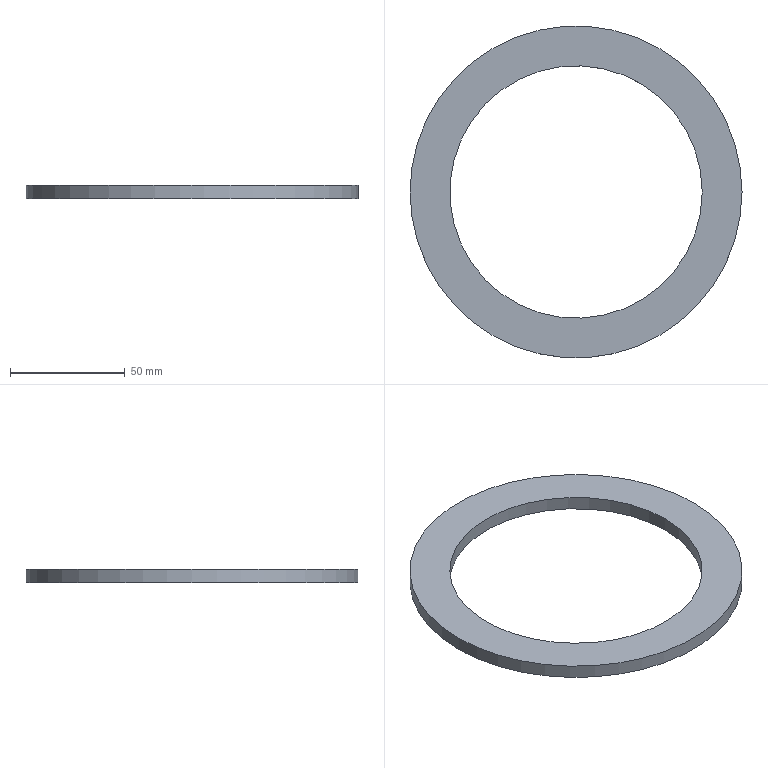Part | NX | features BREP 1 | 1 solid | 4 faces | box 144.7 x 144.7 x 6 mm | volume 41649 mm3 | cylinder 2 | plane 2 | commonest cylinder face diameters 110 x1 144.7 x1
STEP:
#1=CARTESIAN_POINT('',(55.,0.,0.));
#2=VERTEX_POINT('',#1);
#3=CARTESIAN_POINT('',(0.,0.,0.));
#4=DIRECTION('',(0.,0.,1.));
#5=DIRECTION('',(1.,0.,0.));
#6=AXIS2_PLACEMENT_3D('',#3,#4,#5);
#7=CIRCLE('',#6,55.);
#8=EDGE_CURVE('',#2,#2,#7,.T.);
#9=ORIENTED_EDGE('',*,*,#8,.F.);
#10=EDGE_LOOP('',(#9));
#11=FACE_BOUND('',#10,.T.);
#12=CARTESIAN_POINT('',(55.,0.,6.));
#13=VERTEX_POINT('',#12);
#14=CARTESIAN_POINT('',(0.,0.,6.));
#15=DIRECTION('',(0.,0.,1.));
#16=DIRECTION('',(1.,0.,0.));
#17=AXIS2_PLACEMENT_3D('',#14,#15,#16);
#18=CIRCLE('',#17,55.);
#19=EDGE_CURVE('',#13,#13,#18,.T.);
#20=ORIENTED_EDGE('',*,*,#19,.T.);
#21=EDGE_LOOP('',(#20));
#22=FACE_BOUND('',#21,.T.);
#23=CARTESIAN_POINT('',(0.,0.,6.));
#24=DIRECTION('',(0.,0.,-1.));
#25=DIRECTION('',(-1.,0.,0.));
#26=AXIS2_PLACEMENT_3D('',#23,#24,#25);
#27=CYLINDRICAL_SURFACE('',#26,55.);
#28=ADVANCED_FACE('',(#11,#22),#27,.F.);
#29=CARTESIAN_POINT('',(72.35,0.,0.));
#30=VERTEX_POINT('',#29);
#31=CARTESIAN_POINT('',(0.,0.,0.));
#32=DIRECTION('',(0.,0.,1.));
#33=DIRECTION('',(1.,0.,0.));
#34=AXIS2_PLACEMENT_3D('',#31,#32,#33);
#35=CIRCLE('',#34,72.35);
#36=EDGE_CURVE('',#30,#30,#35,.T.);
#37=ORIENTED_EDGE('',*,*,#36,.T.);
#38=EDGE_LOOP('',(#37));
#39=FACE_BOUND('',#38,.T.);
#40=CARTESIAN_POINT('',(72.35,0.,6.));
#41=VERTEX_POINT('',#40);
#42=CARTESIAN_POINT('',(0.,0.,6.));
#43=DIRECTION('',(0.,0.,1.));
#44=DIRECTION('',(1.,0.,0.));
#45=AXIS2_PLACEMENT_3D('',#42,#43,#44);
#46=CIRCLE('',#45,72.35);
#47=EDGE_CURVE('',#41,#41,#46,.T.);
#48=ORIENTED_EDGE('',*,*,#47,.F.);
#49=EDGE_LOOP('',(#48));
#50=FACE_BOUND('',#49,.T.);
#51=CARTESIAN_POINT('',(0.,0.,6.));
#52=DIRECTION('',(0.,0.,-1.));
#53=DIRECTION('',(-1.,0.,0.));
#54=AXIS2_PLACEMENT_3D('',#51,#52,#53);
#55=CYLINDRICAL_SURFACE('',#54,72.35);
#56=ADVANCED_FACE('',(#39,#50),#55,.T.);
#57=ORIENTED_EDGE('',*,*,#47,.T.);
#58=EDGE_LOOP('',(#57));
#59=FACE_BOUND('',#58,.T.);
#60=ORIENTED_EDGE('',*,*,#19,.F.);
#61=EDGE_LOOP('',(#60));
#62=FACE_BOUND('',#61,.T.);
#63=CARTESIAN_POINT('',(0.,0.,6.));
#64=DIRECTION('',(0.,0.,1.));
#65=DIRECTION('',(1.,0.,0.));
#66=AXIS2_PLACEMENT_3D('',#63,#64,#65);
#67=PLANE('',#66);
#68=ADVANCED_FACE('',(#59,#62),#67,.T.);
#69=ORIENTED_EDGE('',*,*,#36,.F.);
#70=EDGE_LOOP('',(#69));
#71=FACE_BOUND('',#70,.T.);
#72=ORIENTED_EDGE('',*,*,#8,.T.);
#73=EDGE_LOOP('',(#72));
#74=FACE_BOUND('',#73,.T.);
#75=CARTESIAN_POINT('',(0.,0.,0.));
#76=DIRECTION('',(0.,0.,1.));
#77=DIRECTION('',(1.,0.,0.));
#78=AXIS2_PLACEMENT_3D('',#75,#76,#77);
#79=PLANE('',#78);
#80=ADVANCED_FACE('',(#71,#74),#79,.F.);
#81=CLOSED_SHELL('',(#28,#56,#68,#80));
#82=MANIFOLD_SOLID_BREP('',#81);
#83=(LENGTH_UNIT()NAMED_UNIT(*)SI_UNIT(.MILLI.,.METRE.));
#84=UNCERTAINTY_MEASURE_WITH_UNIT(LENGTH_MEASURE(0.00001),#83,'','');
#85=(NAMED_UNIT(*)PLANE_ANGLE_UNIT()SI_UNIT($,.RADIAN.));
#86=(NAMED_UNIT(*)SI_UNIT($,.STERADIAN.)SOLID_ANGLE_UNIT());
#87=(GEOMETRIC_REPRESENTATION_CONTEXT(3)GLOBAL_UNCERTAINTY_ASSIGNED_CONTEXT((#84))GLOBAL_UNIT_ASSIGNED_CONTEXT((#83,#85,#86))REPRESENTATION_CONTEXT('',''));
#88=ADVANCED_BREP_SHAPE_REPRESENTATION('',(#82),#87);